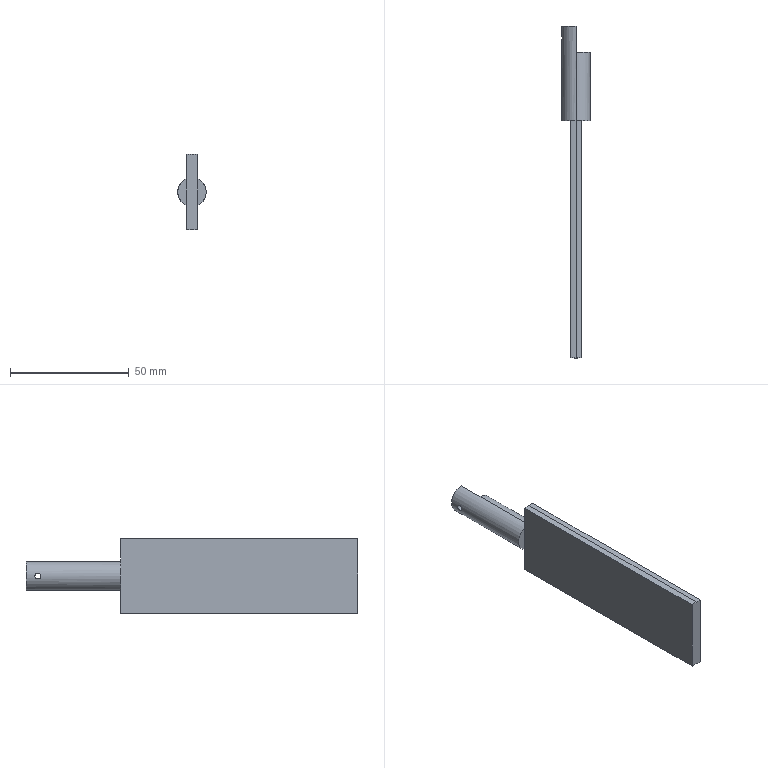Part | SolidWorks | features ICE 3, Extrusion 1, HoleWzd 1 | 1 solid | 19 faces | box 12 x 140 x 32 mm | volume 19807 mm3 | plane 10 | cylinder 7 | cone 2 | commonest cylinder face diameters 32 x3 2.5 x2 12 x2
STEP:
#1=CARTESIAN_POINT('',(-0.275,35.,1.25));
#2=VERTEX_POINT('',#1);
#3=CARTESIAN_POINT('',(-0.275,35.,-1.25));
#4=VERTEX_POINT('',#3);
#5=CARTESIAN_POINT('',(-0.275,35.,0.));
#6=DIRECTION('',(1.,0.,0.));
#7=DIRECTION('',(0.,0.,-1.));
#8=AXIS2_PLACEMENT_3D('',#5,#6,#7);
#9=CIRCLE('',#8,1.25);
#10=EDGE_CURVE('',#2,#4,#9,.T.);
#11=ORIENTED_EDGE('',*,*,#10,.F.);
#12=CARTESIAN_POINT('',(0.,35.,1.525));
#13=VERTEX_POINT('',#12);
#14=CARTESIAN_POINT('',(0.,35.,1.525));
#15=DIRECTION('',(0.7071,0.,0.7071));
#16=VECTOR('',#15,1000.);
#17=LINE('',#14,#16);
#18=EDGE_CURVE('',#2,#13,#17,.T.);
#19=ORIENTED_EDGE('',*,*,#18,.T.);
#20=CARTESIAN_POINT('',(0.,35.,-1.525));
#21=VERTEX_POINT('',#20);
#22=CARTESIAN_POINT('',(0.,35.,0.));
#23=DIRECTION('',(1.,0.,0.));
#24=DIRECTION('',(0.,0.,-1.));
#25=AXIS2_PLACEMENT_3D('',#22,#23,#24);
#26=CIRCLE('',#25,1.525);
#27=EDGE_CURVE('',#13,#21,#26,.T.);
#28=ORIENTED_EDGE('',*,*,#27,.T.);
#29=CARTESIAN_POINT('',(0.,35.,-1.525));
#30=DIRECTION('',(0.7071,0.,-0.7071));
#31=VECTOR('',#30,1000.);
#32=LINE('',#29,#31);
#33=EDGE_CURVE('',#4,#21,#32,.T.);
#34=ORIENTED_EDGE('',*,*,#33,.F.);
#35=EDGE_LOOP('',(#11,#19,#28,#34));
#36=FACE_OUTER_BOUND('',#35,.T.);
#37=CARTESIAN_POINT('',(0.,35.,0.));
#38=DIRECTION('',(1.,0.,0.));
#39=DIRECTION('',(0.,0.,-1.));
#40=AXIS2_PLACEMENT_3D('',#37,#38,#39);
#41=CONICAL_SURFACE('',#40,1.525,0.7854);
#42=ADVANCED_FACE('',(#36),#41,.F.);
#43=CARTESIAN_POINT('',(-5.868,35.,1.25));
#44=VERTEX_POINT('',#43);
#45=CARTESIAN_POINT('',(-5.868,35.,-1.25));
#46=VERTEX_POINT('',#45);
#47=CARTESIAN_POINT('',(-5.868,35.,1.25));
#48=CARTESIAN_POINT('',(-5.868,34.835,1.25));
#49=CARTESIAN_POINT('',(-5.876,34.672,1.217));
#50=CARTESIAN_POINT('',(-5.9,34.37,1.092));
#51=CARTESIAN_POINT('',(-5.917,34.231,0.9988));
#52=CARTESIAN_POINT('',(-5.952,34.001,0.7691));
#53=CARTESIAN_POINT('',(-5.969,33.908,0.63));
#54=CARTESIAN_POINT('',(-5.993,33.783,0.3293));
#55=CARTESIAN_POINT('',(-6.,33.75,0.1648));
#56=CARTESIAN_POINT('',(-6.,33.75,-0.1664));
#57=CARTESIAN_POINT('',(-5.993,33.783,-0.3289));
#58=CARTESIAN_POINT('',(-5.969,33.909,-0.6314));
#59=CARTESIAN_POINT('',(-5.952,34.002,-0.7697));
#60=CARTESIAN_POINT('',(-5.917,34.232,-0.9994));
#61=CARTESIAN_POINT('',(-5.9,34.371,-1.092));
#62=CARTESIAN_POINT('',(-5.876,34.672,-1.217));
#63=CARTESIAN_POINT('',(-5.868,34.836,-1.25));
#64=CARTESIAN_POINT('',(-5.868,35.,-1.25));
#65=B_SPLINE_CURVE_WITH_KNOTS('',3,(#47,#48,#49,#50,#51,#52,#53,#54,#55,#56,#57,#58,#59,#60,#61,#62,#63,#64),.UNSPECIFIED.,.F.,.F.,(4,2,2,2,2,2,2,2,4),(0.005878,0.006368,0.006858,0.007348,0.007837,0.008327,0.008817,0.009307,0.009797),.UNSPECIFIED.);
#66=EDGE_CURVE('',#44,#46,#65,.T.);
#67=ORIENTED_EDGE('',*,*,#66,.F.);
#68=CARTESIAN_POINT('',(0.,35.,1.25));
#69=DIRECTION('',(1.,0.,0.));
#70=VECTOR('',#69,1000.);
#71=LINE('',#68,#70);
#72=EDGE_CURVE('',#44,#2,#71,.T.);
#73=ORIENTED_EDGE('',*,*,#72,.T.);
#74=ORIENTED_EDGE('',*,*,#10,.T.);
#75=CARTESIAN_POINT('',(0.,35.,-1.25));
#76=DIRECTION('',(1.,0.,0.));
#77=VECTOR('',#76,1000.);
#78=LINE('',#75,#77);
#79=EDGE_CURVE('',#46,#4,#78,.T.);
#80=ORIENTED_EDGE('',*,*,#79,.F.);
#81=EDGE_LOOP('',(#67,#73,#74,#80));
#82=FACE_OUTER_BOUND('',#81,.T.);
#83=CARTESIAN_POINT('',(0.,35.,0.));
#84=DIRECTION('',(1.,0.,0.));
#85=DIRECTION('',(0.,0.,-1.));
#86=AXIS2_PLACEMENT_3D('',#83,#84,#85);
#87=CYLINDRICAL_SURFACE('',#86,1.25);
#88=ADVANCED_FACE('',(#82),#87,.F.);
#89=CARTESIAN_POINT('',(0.,29.,-6.));
#90=VERTEX_POINT('',#89);
#91=CARTESIAN_POINT('',(0.,29.,6.));
#92=VERTEX_POINT('',#91);
#93=CARTESIAN_POINT('',(0.,29.,0.));
#94=DIRECTION('',(0.,-1.,0.));
#95=DIRECTION('',(0.,0.,-1.));
#96=AXIS2_PLACEMENT_3D('',#93,#94,#95);
#97=CIRCLE('',#96,6.);
#98=EDGE_CURVE('',#90,#92,#97,.T.);
#99=ORIENTED_EDGE('',*,*,#98,.T.);
#100=CARTESIAN_POINT('',(0.,0.,6.));
#101=VERTEX_POINT('',#100);
#102=CARTESIAN_POINT('',(0.,40.,6.));
#103=DIRECTION('',(0.,-1.,0.));
#104=VECTOR('',#103,1000.);
#105=LINE('',#102,#104);
#106=EDGE_CURVE('',#92,#101,#105,.T.);
#107=ORIENTED_EDGE('',*,*,#106,.T.);
#108=CARTESIAN_POINT('',(2.5,0.,5.454));
#109=VERTEX_POINT('',#108);
#110=CARTESIAN_POINT('',(0.,0.,0.));
#111=DIRECTION('',(0.,1.,0.));
#112=DIRECTION('',(0.,0.,1.));
#113=AXIS2_PLACEMENT_3D('',#110,#111,#112);
#114=CIRCLE('',#113,6.);
#115=EDGE_CURVE('',#101,#109,#114,.T.);
#116=ORIENTED_EDGE('',*,*,#115,.T.);
#117=CARTESIAN_POINT('',(2.5,0.,-5.454));
#118=VERTEX_POINT('',#117);
#119=CARTESIAN_POINT('',(0.,0.,0.));
#120=DIRECTION('',(0.,1.,0.));
#121=DIRECTION('',(0.,0.,1.));
#122=AXIS2_PLACEMENT_3D('',#119,#120,#121);
#123=CIRCLE('',#122,6.);
#124=EDGE_CURVE('',#109,#118,#123,.T.);
#125=ORIENTED_EDGE('',*,*,#124,.T.);
#126=CARTESIAN_POINT('',(0.,0.,-6.));
#127=VERTEX_POINT('',#126);
#128=CARTESIAN_POINT('',(0.,0.,0.));
#129=DIRECTION('',(0.,1.,0.));
#130=DIRECTION('',(0.,0.,1.));
#131=AXIS2_PLACEMENT_3D('',#128,#129,#130);
#132=CIRCLE('',#131,6.);
#133=EDGE_CURVE('',#118,#127,#132,.T.);
#134=ORIENTED_EDGE('',*,*,#133,.T.);
#135=CARTESIAN_POINT('',(0.,40.,-6.));
#136=DIRECTION('',(0.,-1.,0.));
#137=VECTOR('',#136,1000.);
#138=LINE('',#135,#137);
#139=EDGE_CURVE('',#90,#127,#138,.T.);
#140=ORIENTED_EDGE('',*,*,#139,.F.);
#141=EDGE_LOOP('',(#99,#107,#116,#125,#134,#140));
#142=FACE_OUTER_BOUND('',#141,.T.);
#143=CARTESIAN_POINT('',(0.,40.,0.));
#144=DIRECTION('',(0.,-1.,0.));
#145=DIRECTION('',(0.,0.,-1.));
#146=AXIS2_PLACEMENT_3D('',#143,#144,#145);
#147=CYLINDRICAL_SURFACE('',#146,6.);
#148=ADVANCED_FACE('',(#142),#147,.T.);
#149=CARTESIAN_POINT('',(0.,-100.,16.));
#150=VERTEX_POINT('',#149);
#151=CARTESIAN_POINT('',(-2.5,-100.,15.803));
#152=VERTEX_POINT('',#151);
#153=CARTESIAN_POINT('',(0.,-100.,0.));
#154=DIRECTION('',(0.,-1.,0.));
#155=DIRECTION('',(0.,0.,-1.));
#156=AXIS2_PLACEMENT_3D('',#153,#154,#155);
#157=CIRCLE('',#156,16.);
#158=EDGE_CURVE('',#150,#152,#157,.T.);
#159=ORIENTED_EDGE('',*,*,#158,.F.);
#160=CARTESIAN_POINT('',(0.,0.,16.));
#161=VERTEX_POINT('',#160);
#162=CARTESIAN_POINT('',(0.,-100.,16.));
#163=DIRECTION('',(0.,1.,0.));
#164=VECTOR('',#163,1000.);
#165=LINE('',#162,#164);
#166=EDGE_CURVE('',#150,#161,#165,.T.);
#167=ORIENTED_EDGE('',*,*,#166,.T.);
#168=CARTESIAN_POINT('',(-2.5,0.,15.803));
#169=VERTEX_POINT('',#168);
#170=CARTESIAN_POINT('',(0.,0.,0.));
#171=DIRECTION('',(0.,-1.,0.));
#172=DIRECTION('',(0.,0.,-1.));
#173=AXIS2_PLACEMENT_3D('',#170,#171,#172);
#174=CIRCLE('',#173,16.);
#175=EDGE_CURVE('',#161,#169,#174,.T.);
#176=ORIENTED_EDGE('',*,*,#175,.T.);
#177=CARTESIAN_POINT('',(-2.5,-100.,15.803));
#178=DIRECTION('',(0.,1.,0.));
#179=VECTOR('',#178,1000.);
#180=LINE('',#177,#179);
#181=EDGE_CURVE('',#152,#169,#180,.T.);
#182=ORIENTED_EDGE('',*,*,#181,.F.);
#183=EDGE_LOOP('',(#159,#167,#176,#182));
#184=FACE_OUTER_BOUND('',#183,.T.);
#185=CARTESIAN_POINT('',(0.,-100.,0.));
#186=DIRECTION('',(0.,1.,0.));
#187=DIRECTION('',(0.,0.,1.));
#188=AXIS2_PLACEMENT_3D('',#185,#186,#187);
#189=CYLINDRICAL_SURFACE('',#188,16.);
#190=ADVANCED_FACE('',(#184),#189,.T.);
#191=ORIENTED_EDGE('',*,*,#166,.F.);
#192=CARTESIAN_POINT('',(2.5,-100.,15.803));
#193=VERTEX_POINT('',#192);
#194=CARTESIAN_POINT('',(0.,-100.,0.));
#195=DIRECTION('',(0.,-1.,0.));
#196=DIRECTION('',(0.,0.,-1.));
#197=AXIS2_PLACEMENT_3D('',#194,#195,#196);
#198=CIRCLE('',#197,16.);
#199=EDGE_CURVE('',#193,#150,#198,.T.);
#200=ORIENTED_EDGE('',*,*,#199,.F.);
#201=CARTESIAN_POINT('',(2.5,0.,15.803));
#202=VERTEX_POINT('',#201);
#203=CARTESIAN_POINT('',(2.5,-100.,15.803));
#204=DIRECTION('',(0.,-1.,0.));
#205=VECTOR('',#204,1000.);
#206=LINE('',#203,#205);
#207=EDGE_CURVE('',#202,#193,#206,.T.);
#208=ORIENTED_EDGE('',*,*,#207,.F.);
#209=CARTESIAN_POINT('',(0.,0.,0.));
#210=DIRECTION('',(0.,-1.,0.));
#211=DIRECTION('',(0.,0.,-1.));
#212=AXIS2_PLACEMENT_3D('',#209,#210,#211);
#213=CIRCLE('',#212,16.);
#214=EDGE_CURVE('',#202,#161,#213,.T.);
#215=ORIENTED_EDGE('',*,*,#214,.T.);
#216=EDGE_LOOP('',(#191,#200,#208,#215));
#217=FACE_OUTER_BOUND('',#216,.T.);
#218=CARTESIAN_POINT('',(0.,-100.,0.));
#219=DIRECTION('',(0.,1.,0.));
#220=DIRECTION('',(0.,0.,1.));
#221=AXIS2_PLACEMENT_3D('',#218,#219,#220);
#222=CYLINDRICAL_SURFACE('',#221,16.);
#223=ADVANCED_FACE('',(#217),#222,.T.);
#224=CARTESIAN_POINT('',(-2.5,0.,-15.803));
#225=VERTEX_POINT('',#224);
#226=CARTESIAN_POINT('',(-2.5,-100.,-15.803));
#227=VERTEX_POINT('',#226);
#228=CARTESIAN_POINT('',(-2.5,-100.,-15.803));
#229=DIRECTION('',(0.,-1.,0.));
#230=VECTOR('',#229,1000.);
#231=LINE('',#228,#230);
#232=EDGE_CURVE('',#225,#227,#231,.T.);
#233=ORIENTED_EDGE('',*,*,#232,.F.);
#234=CARTESIAN_POINT('',(2.5,0.,-15.803));
#235=VERTEX_POINT('',#234);
#236=CARTESIAN_POINT('',(0.,0.,0.));
#237=DIRECTION('',(0.,-1.,0.));
#238=DIRECTION('',(0.,0.,-1.));
#239=AXIS2_PLACEMENT_3D('',#236,#237,#238);
#240=CIRCLE('',#239,16.);
#241=EDGE_CURVE('',#225,#235,#240,.T.);
#242=ORIENTED_EDGE('',*,*,#241,.T.);
#243=CARTESIAN_POINT('',(2.5,-100.,-15.803));
#244=VERTEX_POINT('',#243);
#245=CARTESIAN_POINT('',(2.5,-100.,-15.803));
#246=DIRECTION('',(0.,1.,0.));
#247=VECTOR('',#246,1000.);
#248=LINE('',#245,#247);
#249=EDGE_CURVE('',#244,#235,#248,.T.);
#250=ORIENTED_EDGE('',*,*,#249,.F.);
#251=CARTESIAN_POINT('',(0.,-100.,0.));
#252=DIRECTION('',(0.,-1.,0.));
#253=DIRECTION('',(0.,0.,-1.));
#254=AXIS2_PLACEMENT_3D('',#251,#252,#253);
#255=CIRCLE('',#254,16.);
#256=EDGE_CURVE('',#227,#244,#255,.T.);
#257=ORIENTED_EDGE('',*,*,#256,.F.);
#258=EDGE_LOOP('',(#233,#242,#250,#257));
#259=FACE_OUTER_BOUND('',#258,.T.);
#260=CARTESIAN_POINT('',(0.,-100.,0.));
#261=DIRECTION('',(0.,1.,0.));
#262=DIRECTION('',(0.,0.,1.));
#263=AXIS2_PLACEMENT_3D('',#260,#261,#262);
#264=CYLINDRICAL_SURFACE('',#263,16.);
#265=ADVANCED_FACE('',(#259),#264,.T.);
#266=ORIENTED_EDGE('',*,*,#199,.T.);
#267=ORIENTED_EDGE('',*,*,#158,.T.);
#268=CARTESIAN_POINT('',(-2.5,-100.,0.));
#269=DIRECTION('',(0.,0.,-1.));
#270=VECTOR('',#269,1000.);
#271=LINE('',#268,#270);
#272=EDGE_CURVE('',#152,#227,#271,.T.);
#273=ORIENTED_EDGE('',*,*,#272,.T.);
#274=ORIENTED_EDGE('',*,*,#256,.T.);
#275=CARTESIAN_POINT('',(2.5,-100.,0.));
#276=DIRECTION('',(0.,0.,1.));
#277=VECTOR('',#276,1000.);
#278=LINE('',#275,#277);
#279=EDGE_CURVE('',#244,#193,#278,.T.);
#280=ORIENTED_EDGE('',*,*,#279,.T.);
#281=EDGE_LOOP('',(#266,#267,#273,#274,#280));
#282=FACE_OUTER_BOUND('',#281,.T.);
#283=CARTESIAN_POINT('',(0.,-100.,0.));
#284=DIRECTION('',(0.,-1.,0.));
#285=DIRECTION('',(0.,0.,-1.));
#286=AXIS2_PLACEMENT_3D('',#283,#284,#285);
#287=PLANE('',#286);
#288=ADVANCED_FACE('',(#282),#287,.T.);
#289=CARTESIAN_POINT('',(-2.5,0.,5.454));
#290=VERTEX_POINT('',#289);
#291=CARTESIAN_POINT('',(-2.5,0.,0.));
#292=DIRECTION('',(0.,0.,-1.));
#293=VECTOR('',#292,1000.);
#294=LINE('',#291,#293);
#295=EDGE_CURVE('',#169,#290,#294,.T.);
#296=ORIENTED_EDGE('',*,*,#295,.F.);
#297=ORIENTED_EDGE('',*,*,#175,.F.);
#298=ORIENTED_EDGE('',*,*,#214,.F.);
#299=CARTESIAN_POINT('',(2.5,0.,0.));
#300=DIRECTION('',(0.,0.,1.));
#301=VECTOR('',#300,1000.);
#302=LINE('',#299,#301);
#303=EDGE_CURVE('',#109,#202,#302,.T.);
#304=ORIENTED_EDGE('',*,*,#303,.F.);
#305=ORIENTED_EDGE('',*,*,#115,.F.);
#306=CARTESIAN_POINT('',(0.,0.,0.));
#307=DIRECTION('',(0.,1.,0.));
#308=DIRECTION('',(0.,0.,1.));
#309=AXIS2_PLACEMENT_3D('',#306,#307,#308);
#310=CIRCLE('',#309,6.);
#311=EDGE_CURVE('',#290,#101,#310,.T.);
#312=ORIENTED_EDGE('',*,*,#311,.F.);
#313=EDGE_LOOP('',(#296,#297,#298,#304,#305,#312));
#314=FACE_OUTER_BOUND('',#313,.T.);
#315=CARTESIAN_POINT('',(0.,0.,0.));
#316=DIRECTION('',(0.,-1.,0.));
#317=DIRECTION('',(0.,0.,-1.));
#318=AXIS2_PLACEMENT_3D('',#315,#316,#317);
#319=PLANE('',#318);
#320=ADVANCED_FACE('',(#314),#319,.F.);
#321=CARTESIAN_POINT('',(-2.5,0.,-5.454));
#322=VERTEX_POINT('',#321);
#323=CARTESIAN_POINT('',(-2.5,0.,0.));
#324=DIRECTION('',(0.,0.,-1.));
#325=VECTOR('',#324,1000.);
#326=LINE('',#323,#325);
#327=EDGE_CURVE('',#322,#225,#326,.T.);
#328=ORIENTED_EDGE('',*,*,#327,.F.);
#329=CARTESIAN_POINT('',(0.,0.,0.));
#330=DIRECTION('',(0.,1.,0.));
#331=DIRECTION('',(0.,0.,1.));
#332=AXIS2_PLACEMENT_3D('',#329,#330,#331);
#333=CIRCLE('',#332,6.);
#334=EDGE_CURVE('',#127,#322,#333,.T.);
#335=ORIENTED_EDGE('',*,*,#334,.F.);
#336=ORIENTED_EDGE('',*,*,#133,.F.);
#337=CARTESIAN_POINT('',(2.5,0.,0.));
#338=DIRECTION('',(0.,0.,1.));
#339=VECTOR('',#338,1000.);
#340=LINE('',#337,#339);
#341=EDGE_CURVE('',#235,#118,#340,.T.);
#342=ORIENTED_EDGE('',*,*,#341,.F.);
#343=ORIENTED_EDGE('',*,*,#241,.F.);
#344=EDGE_LOOP('',(#328,#335,#336,#342,#343));
#345=FACE_OUTER_BOUND('',#344,.T.);
#346=CARTESIAN_POINT('',(0.,0.,0.));
#347=DIRECTION('',(0.,-1.,0.));
#348=DIRECTION('',(0.,0.,-1.));
#349=AXIS2_PLACEMENT_3D('',#346,#347,#348);
#350=PLANE('',#349);
#351=ADVANCED_FACE('',(#345),#350,.F.);
#352=ORIENTED_EDGE('',*,*,#106,.F.);
#353=CARTESIAN_POINT('',(0.,40.,6.));
#354=VERTEX_POINT('',#353);
#355=CARTESIAN_POINT('',(0.,40.,6.));
#356=DIRECTION('',(0.,-1.,0.));
#357=VECTOR('',#356,1000.);
#358=LINE('',#355,#357);
#359=EDGE_CURVE('',#354,#92,#358,.T.);
#360=ORIENTED_EDGE('',*,*,#359,.F.);
#361=CARTESIAN_POINT('',(0.,40.,-6.));
#362=VERTEX_POINT('',#361);
#363=CARTESIAN_POINT('',(0.,40.,0.));
#364=DIRECTION('',(0.,1.,0.));
#365=DIRECTION('',(0.,0.,1.));
#366=AXIS2_PLACEMENT_3D('',#363,#364,#365);
#367=CIRCLE('',#366,6.);
#368=EDGE_CURVE('',#362,#354,#367,.T.);
#369=ORIENTED_EDGE('',*,*,#368,.F.);
#370=CARTESIAN_POINT('',(0.,40.,-6.));
#371=DIRECTION('',(0.,-1.,0.));
#372=VECTOR('',#371,1000.);
#373=LINE('',#370,#372);
#374=EDGE_CURVE('',#362,#90,#373,.T.);
#375=ORIENTED_EDGE('',*,*,#374,.T.);
#376=ORIENTED_EDGE('',*,*,#139,.T.);
#377=ORIENTED_EDGE('',*,*,#334,.T.);
#378=CARTESIAN_POINT('',(0.,0.,0.));
#379=DIRECTION('',(0.,1.,0.));
#380=DIRECTION('',(0.,0.,1.));
#381=AXIS2_PLACEMENT_3D('',#378,#379,#380);
#382=CIRCLE('',#381,6.);
#383=EDGE_CURVE('',#322,#290,#382,.T.);
#384=ORIENTED_EDGE('',*,*,#383,.T.);
#385=ORIENTED_EDGE('',*,*,#311,.T.);
#386=EDGE_LOOP('',(#352,#360,#369,#375,#376,#377,#384,#385));
#387=FACE_OUTER_BOUND('',#386,.T.);
#388=CARTESIAN_POINT('',(-5.868,35.,-1.25));
#389=CARTESIAN_POINT('',(-5.868,35.082,-1.25));
#390=CARTESIAN_POINT('',(-5.87,35.165,-1.242));
#391=CARTESIAN_POINT('',(-5.877,35.325,-1.21));
#392=CARTESIAN_POINT('',(-5.882,35.403,-1.186));
#393=CARTESIAN_POINT('',(-5.9,35.631,-1.092));
#394=CARTESIAN_POINT('',(-5.917,35.768,-0.9997));
#395=CARTESIAN_POINT('',(-5.952,36.,-0.7674));
#396=CARTESIAN_POINT('',(-5.969,36.092,-0.6296));
#397=CARTESIAN_POINT('',(-5.993,36.217,-0.3275));
#398=CARTESIAN_POINT('',(-6.,36.25,-0.1631));
#399=CARTESIAN_POINT('',(-6.,36.25,0.1637));
#400=CARTESIAN_POINT('',(-5.993,36.217,0.3286));
#401=CARTESIAN_POINT('',(-5.969,36.092,0.6296));
#402=CARTESIAN_POINT('',(-5.952,35.999,0.7684));
#403=CARTESIAN_POINT('',(-5.917,35.769,0.999));
#404=CARTESIAN_POINT('',(-5.9,35.631,1.091));
#405=CARTESIAN_POINT('',(-5.876,35.328,1.217));
#406=CARTESIAN_POINT('',(-5.868,35.165,1.25));
#407=CARTESIAN_POINT('',(-5.868,35.,1.25));
#408=B_SPLINE_CURVE_WITH_KNOTS('',3,(#388,#389,#390,#391,#392,#393,#394,#395,#396,#397,#398,#399,#400,#401,#402,#403,#404,#405,#406,#407),.UNSPECIFIED.,.F.,.F.,(4,2,2,2,2,2,2,2,2,4),(0.00196,0.002205,0.00245,0.00294,0.003429,0.003919,0.004409,0.004899,0.005389,0.005878),.UNSPECIFIED.);
#409=EDGE_CURVE('',#46,#44,#408,.T.);
#410=ORIENTED_EDGE('',*,*,#409,.T.);
#411=ORIENTED_EDGE('',*,*,#66,.T.);
#412=EDGE_LOOP('',(#410,#411));
#413=FACE_BOUND('',#412,.T.);
#414=CARTESIAN_POINT('',(0.,40.,0.));
#415=DIRECTION('',(0.,-1.,0.));
#416=DIRECTION('',(0.,0.,-1.));
#417=AXIS2_PLACEMENT_3D('',#414,#415,#416);
#418=CYLINDRICAL_SURFACE('',#417,6.);
#419=ADVANCED_FACE('',(#387,#413),#418,.T.);
#420=CARTESIAN_POINT('',(0.,40.,-6.));
#421=DIRECTION('',(0.,0.,1.));
#422=VECTOR('',#421,1000.);
#423=LINE('',#420,#422);
#424=EDGE_CURVE('',#362,#354,#423,.T.);
#425=ORIENTED_EDGE('',*,*,#424,.F.);
#426=ORIENTED_EDGE('',*,*,#368,.T.);
#427=EDGE_LOOP('',(#425,#426));
#428=FACE_OUTER_BOUND('',#427,.T.);
#429=CARTESIAN_POINT('',(0.,40.,0.));
#430=DIRECTION('',(0.,1.,0.));
#431=DIRECTION('',(0.,0.,1.));
#432=AXIS2_PLACEMENT_3D('',#429,#430,#431);
#433=PLANE('',#432);
#434=ADVANCED_FACE('',(#428),#433,.T.);
#435=CARTESIAN_POINT('',(0.,29.,-6.));
#436=DIRECTION('',(0.,0.,1.));
#437=VECTOR('',#436,1000.);
#438=LINE('',#435,#437);
#439=EDGE_CURVE('',#90,#92,#438,.T.);
#440=ORIENTED_EDGE('',*,*,#439,.T.);
#441=ORIENTED_EDGE('',*,*,#98,.F.);
#442=EDGE_LOOP('',(#440,#441));
#443=FACE_OUTER_BOUND('',#442,.T.);
#444=CARTESIAN_POINT('',(0.,29.,-6.));
#445=DIRECTION('',(0.,-1.,0.));
#446=DIRECTION('',(0.,0.,-1.));
#447=AXIS2_PLACEMENT_3D('',#444,#445,#446);
#448=PLANE('',#447);
#449=ADVANCED_FACE('',(#443),#448,.F.);
#450=CARTESIAN_POINT('',(0.,35.,0.));
#451=DIRECTION('',(1.,0.,0.));
#452=DIRECTION('',(0.,0.,-1.));
#453=AXIS2_PLACEMENT_3D('',#450,#451,#452);
#454=CIRCLE('',#453,1.525);
#455=EDGE_CURVE('',#21,#13,#454,.T.);
#456=ORIENTED_EDGE('',*,*,#455,.F.);
#457=ORIENTED_EDGE('',*,*,#27,.F.);
#458=EDGE_LOOP('',(#456,#457));
#459=FACE_BOUND('',#458,.T.);
#460=ORIENTED_EDGE('',*,*,#439,.F.);
#461=ORIENTED_EDGE('',*,*,#374,.F.);
#462=ORIENTED_EDGE('',*,*,#424,.T.);
#463=ORIENTED_EDGE('',*,*,#359,.T.);
#464=EDGE_LOOP('',(#460,#461,#462,#463));
#465=FACE_OUTER_BOUND('',#464,.T.);
#466=CARTESIAN_POINT('',(0.,40.,-6.));
#467=DIRECTION('',(-1.,0.,0.));
#468=DIRECTION('',(0.,-1.,0.));
#469=AXIS2_PLACEMENT_3D('',#466,#467,#468);
#470=PLANE('',#469);
#471=ADVANCED_FACE('',(#459,#465),#470,.F.);
#472=ORIENTED_EDGE('',*,*,#72,.F.);
#473=ORIENTED_EDGE('',*,*,#409,.F.);
#474=ORIENTED_EDGE('',*,*,#79,.T.);
#475=CARTESIAN_POINT('',(-0.275,35.,0.));
#476=DIRECTION('',(1.,0.,0.));
#477=DIRECTION('',(0.,0.,-1.));
#478=AXIS2_PLACEMENT_3D('',#475,#476,#477);
#479=CIRCLE('',#478,1.25);
#480=EDGE_CURVE('',#4,#2,#479,.T.);
#481=ORIENTED_EDGE('',*,*,#480,.T.);
#482=EDGE_LOOP('',(#472,#473,#474,#481));
#483=FACE_OUTER_BOUND('',#482,.T.);
#484=CARTESIAN_POINT('',(0.,35.,0.));
#485=DIRECTION('',(1.,0.,0.));
#486=DIRECTION('',(0.,0.,-1.));
#487=AXIS2_PLACEMENT_3D('',#484,#485,#486);
#488=CYLINDRICAL_SURFACE('',#487,1.25);
#489=ADVANCED_FACE('',(#483),#488,.F.);
#490=ORIENTED_EDGE('',*,*,#18,.F.);
#491=ORIENTED_EDGE('',*,*,#480,.F.);
#492=ORIENTED_EDGE('',*,*,#33,.T.);
#493=ORIENTED_EDGE('',*,*,#455,.T.);
#494=EDGE_LOOP('',(#490,#491,#492,#493));
#495=FACE_OUTER_BOUND('',#494,.T.);
#496=CARTESIAN_POINT('',(0.,35.,0.));
#497=DIRECTION('',(1.,0.,0.));
#498=DIRECTION('',(0.,0.,-1.));
#499=AXIS2_PLACEMENT_3D('',#496,#497,#498);
#500=CONICAL_SURFACE('',#499,1.525,0.7854);
#501=ADVANCED_FACE('',(#495),#500,.F.);
#502=ORIENTED_EDGE('',*,*,#249,.T.);
#503=ORIENTED_EDGE('',*,*,#341,.T.);
#504=CARTESIAN_POINT('',(2.5,0.,20.213));
#505=DIRECTION('',(0.,0.,-1.));
#506=VECTOR('',#505,1000.);
#507=LINE('',#504,#506);
#508=EDGE_CURVE('',#109,#118,#507,.T.);
#509=ORIENTED_EDGE('',*,*,#508,.F.);
#510=ORIENTED_EDGE('',*,*,#303,.T.);
#511=ORIENTED_EDGE('',*,*,#207,.T.);
#512=ORIENTED_EDGE('',*,*,#279,.F.);
#513=EDGE_LOOP('',(#502,#503,#509,#510,#511,#512));
#514=FACE_OUTER_BOUND('',#513,.T.);
#515=CARTESIAN_POINT('',(2.5,52.073,20.213));
#516=DIRECTION('',(1.,0.,0.));
#517=DIRECTION('',(0.,0.,-1.));
#518=AXIS2_PLACEMENT_3D('',#515,#516,#517);
#519=PLANE('',#518);
#520=ADVANCED_FACE('',(#514),#519,.T.);
#521=ORIENTED_EDGE('',*,*,#124,.F.);
#522=ORIENTED_EDGE('',*,*,#508,.T.);
#523=EDGE_LOOP('',(#521,#522));
#524=FACE_OUTER_BOUND('',#523,.T.);
#525=CARTESIAN_POINT('',(0.,0.,0.));
#526=DIRECTION('',(0.,-1.,0.));
#527=DIRECTION('',(0.,0.,-1.));
#528=AXIS2_PLACEMENT_3D('',#525,#526,#527);
#529=PLANE('',#528);
#530=ADVANCED_FACE('',(#524),#529,.T.);
#531=ORIENTED_EDGE('',*,*,#383,.F.);
#532=CARTESIAN_POINT('',(-2.5,0.,20.213));
#533=DIRECTION('',(0.,0.,1.));
#534=VECTOR('',#533,1000.);
#535=LINE('',#532,#534);
#536=EDGE_CURVE('',#322,#290,#535,.T.);
#537=ORIENTED_EDGE('',*,*,#536,.T.);
#538=EDGE_LOOP('',(#531,#537));
#539=FACE_OUTER_BOUND('',#538,.T.);
#540=CARTESIAN_POINT('',(0.,0.,0.));
#541=DIRECTION('',(0.,-1.,0.));
#542=DIRECTION('',(0.,0.,-1.));
#543=AXIS2_PLACEMENT_3D('',#540,#541,#542);
#544=PLANE('',#543);
#545=ADVANCED_FACE('',(#539),#544,.T.);
#546=ORIENTED_EDGE('',*,*,#181,.T.);
#547=ORIENTED_EDGE('',*,*,#295,.T.);
#548=ORIENTED_EDGE('',*,*,#536,.F.);
#549=ORIENTED_EDGE('',*,*,#327,.T.);
#550=ORIENTED_EDGE('',*,*,#232,.T.);
#551=ORIENTED_EDGE('',*,*,#272,.F.);
#552=EDGE_LOOP('',(#546,#547,#548,#549,#550,#551));
#553=FACE_OUTER_BOUND('',#552,.T.);
#554=CARTESIAN_POINT('',(-2.5,52.073,20.213));
#555=DIRECTION('',(-1.,0.,0.));
#556=DIRECTION('',(0.,0.,1.));
#557=AXIS2_PLACEMENT_3D('',#554,#555,#556);
#558=PLANE('',#557);
#559=ADVANCED_FACE('',(#553),#558,.T.);
#560=CLOSED_SHELL('',(#42,#88,#148,#190,#223,#265,#288,#320,#351,#419,#434,#449,#471,#489,#501,#520,#530,#545,#559));
#561=MANIFOLD_SOLID_BREP('',#560);
#562=CARTESIAN_POINT('',(0.,0.,0.));
#563=DIRECTION('',(0.,0.,1.));
#564=DIRECTION('',(1.,0.,0.));
#565=AXIS2_PLACEMENT_3D('',#562,#563,#564);
#566=(LENGTH_UNIT()NAMED_UNIT(*)SI_UNIT(.MILLI.,.METRE.));
#567=UNCERTAINTY_MEASURE_WITH_UNIT(LENGTH_MEASURE(0.00001),#566,'','');
#568=(NAMED_UNIT(*)PLANE_ANGLE_UNIT()SI_UNIT($,.RADIAN.));
#569=(NAMED_UNIT(*)SI_UNIT($,.STERADIAN.)SOLID_ANGLE_UNIT());
#570=(GEOMETRIC_REPRESENTATION_CONTEXT(3)GLOBAL_UNCERTAINTY_ASSIGNED_CONTEXT((#567))GLOBAL_UNIT_ASSIGNED_CONTEXT((#566,#568,#569))REPRESENTATION_CONTEXT('',''));
#571=ADVANCED_BREP_SHAPE_REPRESENTATION('',(#561,#565),#570);